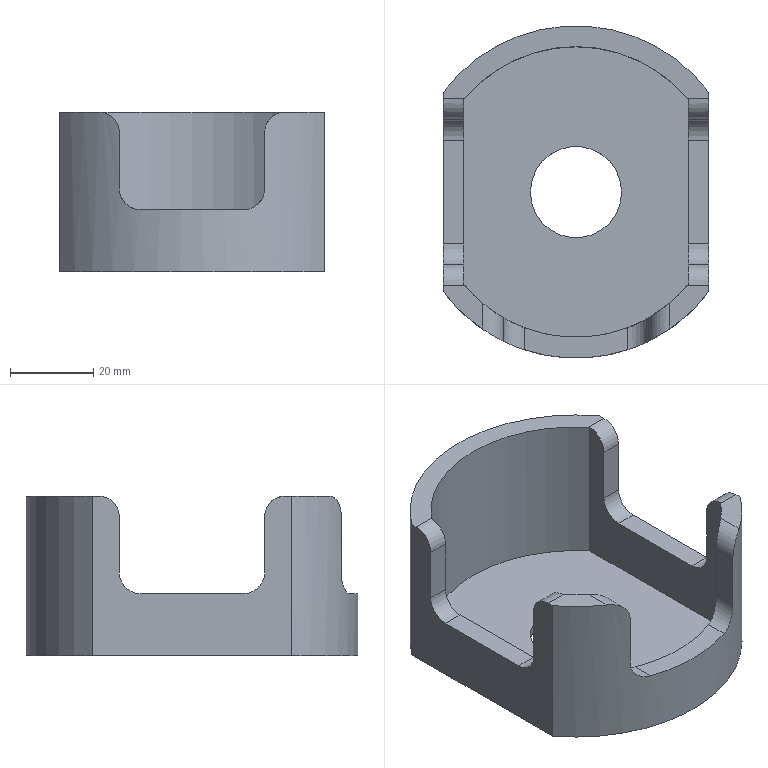Part | STEP file | 1 solid | 36 faces | box 64 x 80 x 38.5 mm | volume 37425 mm3 | cylinder 18 | plane 18 | commonest cylinder face diameters 10 x12 22 x2 70 x2 80 x2